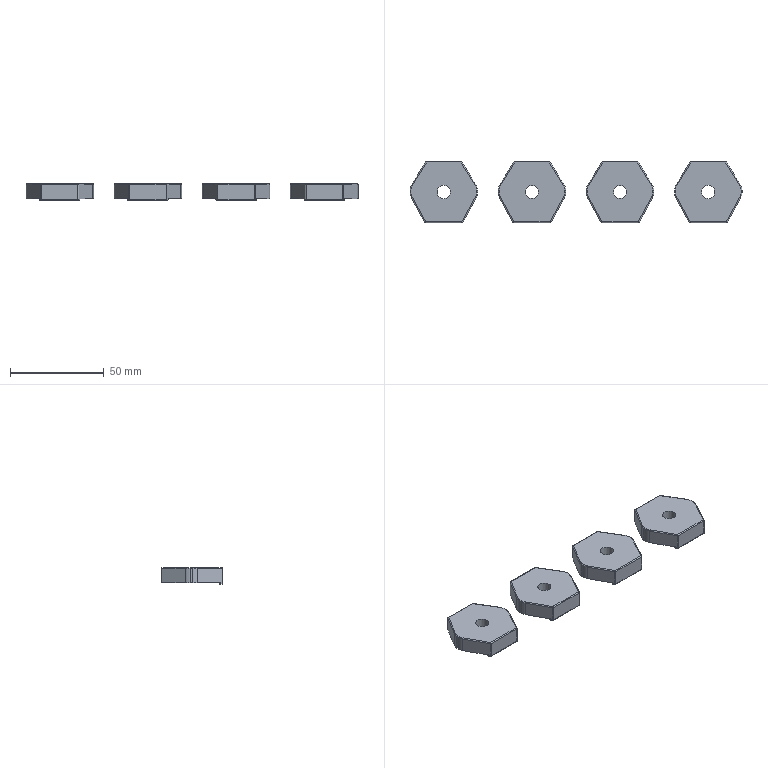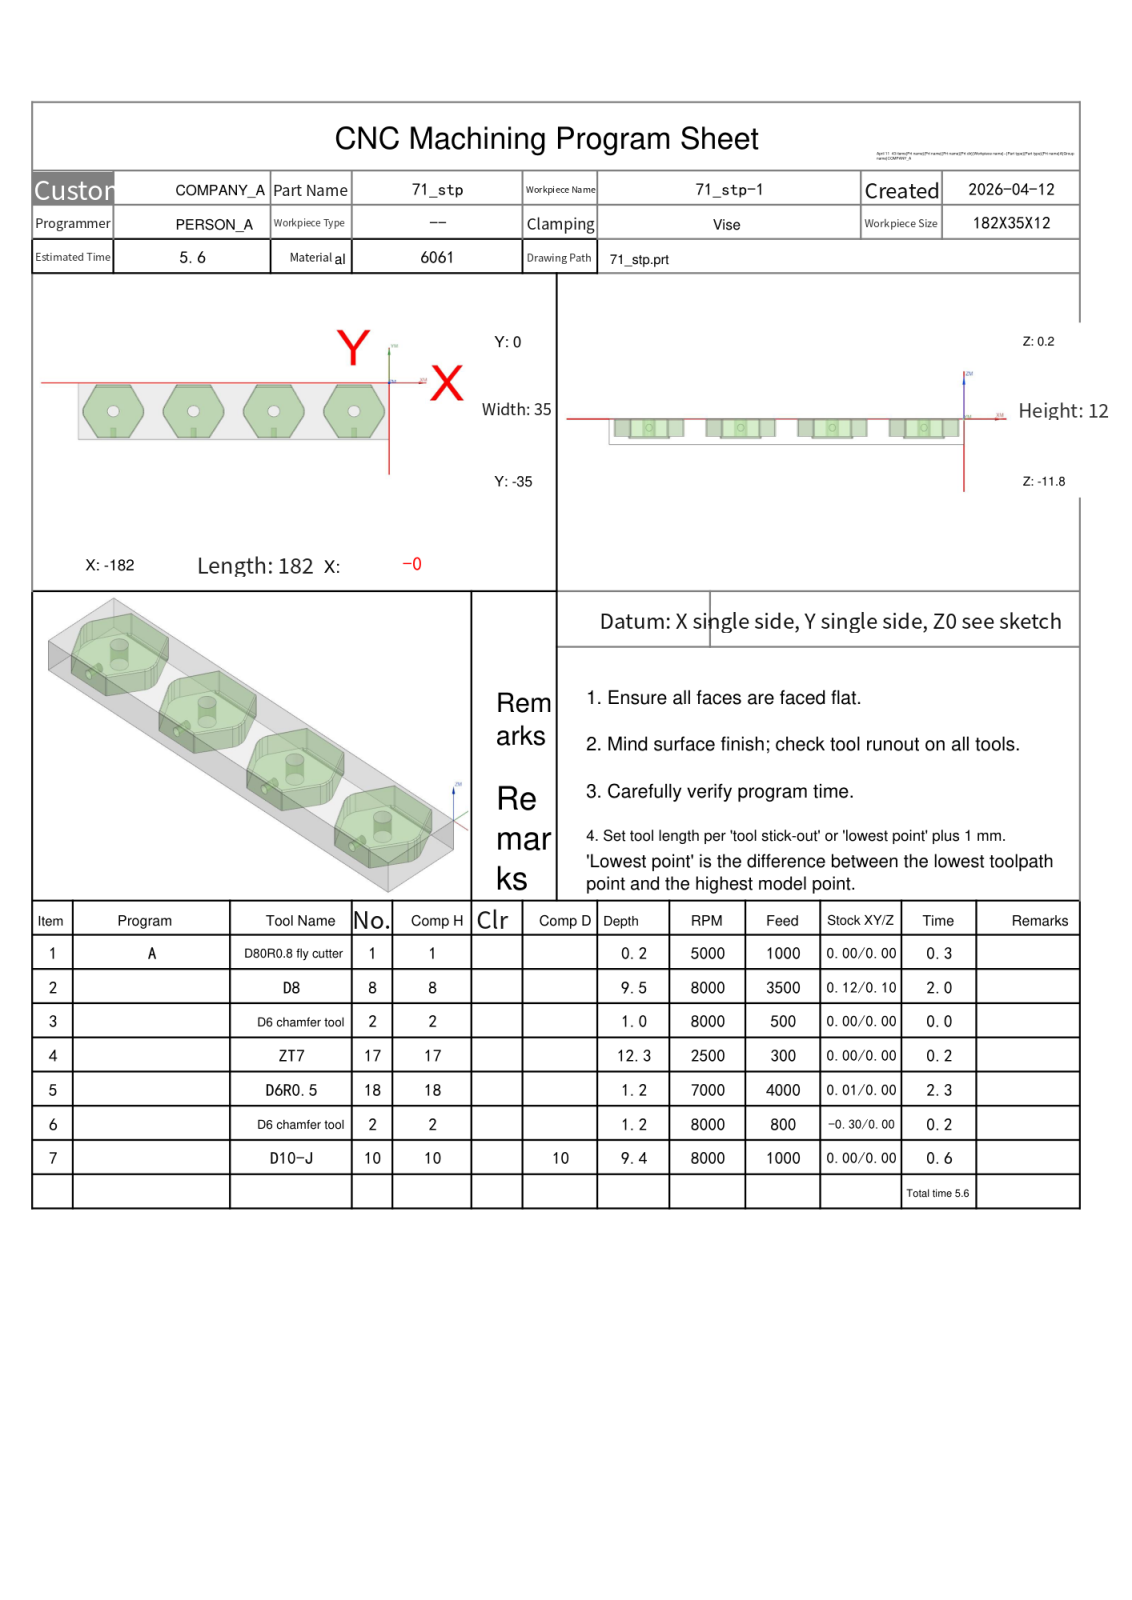NC program | NX | posted by the shop | part box 177 x 33 x 9 mm
Lines 34 to 853 of 15773:
N2 T08 M06
(D8  D=8. R=0. H=08 ce=0.12 di=0.10)
(MAX_Z=20. MIN_Z=-9.3 Time=2.03M)
G00 G90 G54 X-46.469 Y9.631 M03 S8000
G43 H08 Z20.
M08
Z-7.3
G01 X-46.451 Y9.533 Z-7.925 F3500.
X-46.433 Y9.435 Z-8.172
X-46.415 Y9.336 Z-8.354
X-46.396 Y9.238 Z-8.5
X-46.378 Y9.14 Z-8.623
X-46.36 Y9.041 Z-8.728
X-46.342 Y8.943 Z-8.82
X-46.324 Y8.845 Z-8.9
X-46.306 Y8.746 Z-8.97
X-46.287 Y8.648 Z-9.032
X-46.269 Y8.55 Z-9.086
X-46.251 Y8.451 Z-9.133
X-46.233 Y8.353 Z-9.174
X-46.215 Y8.255 Z-9.208
X-46.196 Y8.156 Z-9.236
X-46.178 Y8.058 Z-9.26
X-46.16 Y7.96 Z-9.277
X-46.142 Y7.861 Z-9.29
X-46.124 Y7.763 Z-9.297
X-46.105 Y7.665 Z-9.3
X-45.763 Y5.813
G03 X-45.53 Y5.517 I.405 J.08
X-42.414 Y5.012 I3.116 J9.363
G01 X-42.391
G03 X-34.679 Y4.895 I7.712 J253.536
X-32.981 Y4.9 I0.0 J253.653
G01 X-1.242 Y4.876
G02 X3.834 Y1.179 I-.204 J-5.613
X4.791 Y-4.109 I-15.027 J-5.451
X4.904 Y-11.94 I-270.442 J-7.831
X4.899 Y-13.588 I-270.556 J0.0
G01 X4.875 Y-33.767
G02 X1.064 Y-38.883 I-5.648 J.229
X-4.293 Y-39.8 I-5.462 J15.805
X-12.747 Y-39.907 I-8.454 J336.448
X-14.912 Y-39.9 I0.0 J336.554
G01 X-180.771 Y-39.875
G02 X-185.907 Y-36.005 I.244 J5.667
X-186.809 Y-30.524 I16.45 J5.52
X-186.9 Y-22.424 I358.144 J8.1
G01 X-186.899 Y-21.585
X-186.875 Y-1.225
G02 X-183.098 Y3.867 I5.635 J-.233
X-177.983 Y4.786 I5.357 J-15.119
X-169.888 Y4.907 I8.095 J-270.155
X-167.845 Y4.9 I0.0 J-270.276
G01 X-47.525 Y4.88
G03 X-36.07 Y4.289 I11.455 J110.869
X-34.358 Y4.303 I0.0 J111.459
G01 X-2.782 Y4.281
G02 X2.822 Y.462 I-.263 J-6.407
X4.101 Y-4.997 I-13.81 J-6.115
X4.319 Y-13.515 I-166.113 J-8.518
X4.299 Y-16.093 I-166.332 J0.0
G01 X4.273 Y-32.337
G02 X.456 Y-37.826 I-6.395 J.376
X-5.129 Y-39.111 I-6.168 J14.022
X-12.99 Y-39.311 I-7.861 J154.538
X-14.965 Y-39.298 I0.0 J154.738
G01 X-179.157 Y-39.283
G02 X-184.769 Y-35.572 I.183 J6.375
X-186.101 Y-30.002 I13.537 J6.183
X-186.313 Y-22.099 I147.476 J7.903
X-186.298 Y-20.047 I147.688 J0.0
X-186.324 Y-13.199 I932.526 J6.848
X-186.262 Y-2.503 I932.551 J0.0
X-182.47 Y2.818 I6.388 J-.54
X-176.892 Y4.109 I6.166 J-13.933
X-169.368 Y4.307 I7.524 J-142.898
X-167.716 Y4.298 I0.0 J-143.096
G01 X-48.656 Y4.275
G03 X-39.564 Y3.768 I19.57 J268.931
X-28.389 Y3.691 I11.176 J810.309
X-24.341 Y3.701 I0.0 J810.386
G01 X-4.162 Y3.679
G02 X2.13 Y-.639 I-.299 J-7.178
X3.495 Y-6.63 I-15.458 J-6.673
X3.71 Y-14.745 I-153.347 J-8.114
X3.698 Y-16.646 I-153.562 J0.0
X3.721 Y-22.166 I-646.386 J-5.52
X3.659 Y-31.125 I-646.409 J0.0
X-.568 Y-37.095 I-7.136 J.57
X-6.434 Y-38.479 I-6.628 J14.972
X-13.995 Y-38.704 I-7.56 J127.23
X-15.429 Y-38.695 I0.0 J127.454
G01 X-177.869 Y-38.676
G02 X-184.121 Y-34.381 I.319 J7.163
X-185.493 Y-28.391 I15.365 J6.672
X-185.711 Y-20.229 I153.286 J8.162
X-185.698 Y-18.255 I153.503 J0.0
X-185.723 Y-12.675 I620.518 J5.58
X-185.661 Y-3.896 I620.543 J0.0
X-181.441 Y2.091 I7.135 J-.548
X-175.399 Y3.493 I6.719 J-15.24
X-166.669 Y3.717 I8.73 J-169.523
X-164.123 Y3.698 I0.0 J-169.748
G01 X-49.623 Y3.675
G03 X-39.795 Y3.188 I46.086 J829.839
X-31.558 Y3.118 I8.237 J488.664
X-30.201 Y3.12 I0.0 J488.733
G01 X-5.734 Y3.089
X-5.73
G02 X1.522 Y-1.766 I0.0 J-7.844
X2.883 Y-7.949 I-16.932 J-6.968
X3.108 Y-16.247 I-153.023 J-8.298
X3.097 Y-18.084 I-153.248 J0.0
X3.116 Y-22.347 I-475.2 J-4.263
X3.058 Y-29.803 I-475.219 J0.0
X-1.706 Y-36.495 I-7.774 J.493
X-7.759 Y-37.868 I-6.923 J16.481
G01 X-10.659 Y-38.024
X-11.409 Y-38.12
X-175.683 Y-38.099
G02 X-176.12 Y-38.11 I-.437 J8.29
X-180.889 Y-36.604 I0.0 J8.302
X-184.211 Y-31.307 I5.976 J7.44
X-185.028 Y-24.203 I30.504 J7.104
G01 Y-24.17
G02 X-185.104 Y-13.157 I791.672 J11.013
X-185.065 Y-5.311 I791.749 J0.0
X-180.404 Y1.443 I7.76 J-.37
X-174.182 Y2.874 I7.039 J-16.362
G03 X-171.201 Y3.12 I-1.365 J34.726
G01 X-51.578 Y3.094
G02 X-41.401 Y2.65 I-11.338 J-376.674
G03 X-33.711 Y2.531 I7.69 J247.054
X-32.415 Y2.534 I0.0 J247.174
G02 X-30.298 Y3.107 I2.291 J-4.269
G03 X-32.525 Y2.487 I.219 J-5.098
G02 X-35.859 Y2.103 I-3.334 J14.267
X-36.319 Y2.11 I0.0 J14.652
X-48.557 Y2.523 I1.1 J213.807
G03 X-55.859 Y2.651 I-13.9 J-588.103
G01 X-56.551 Y2.949
X-57.767 Y3.12
G02 X-55.511 Y2.513 I-.263 J-5.475
G03 X-51.539 Y2.054 I4.131 J18.358
X-38.068 Y1.524 I23.165 J416.613
X-37.143 Y1.504 I.925 J21.92
X-33.407 Y1.825 I0.0 J21.939
G01 X-32.511 Y2.493
G02 X-33.72 Y1.652 I-4.216 J4.773
X-37.466 Y1.106 I-3.746 J12.559
X-37.794 Y1.11 I0.0 J13.106
X-49.056 Y1.461 I.153 J185.526
X-54.688 Y1.939 I.335 J37.41
X-55.421 Y2.462 I1.246 J2.524
G01 X-55.642 Y2.557
G02 X-54.763 Y1.937 I-1.218 J-2.657
G03 X-52.007 Y1.171 I3.286 J6.483
X-39.733 Y.542 I12.274 J119.512
X-37.401 Y.565 I0.0 J120.141
X-33.962 Y1.165 I-.011 J10.218
G01 X-33.535 Y1.7
X-33.347 Y1.849
G03 X-33.938 Y1.159 I1.796 J-2.136
G02 X-36.449 Y.31 I-2.939 J4.559
X-41.066 Y.075 I-4.617 J45.074
X-43.901 Y.163 I0.0 J45.309
X-52.223 Y.776 I1.511 J77.385
X-54.179 Y1.336 I1.063 J7.401
G03 X-54.789 Y1.957 I-2.181 J-1.534
G02 X-54.168 Y1.3 I-1.237 J-1.791
G03 X-51.671 Y.286 I3.24 J4.394
X-43.374 Y-.438 I8.951 J54.711
X-41.177 Y-.505 I2.196 J35.678
X-36.411 Y-.186 I0.0 J35.745
X-34.391 Y.502 I-.758 J5.538
G01 X-33.874 Y1.235
G02 X-34.512 Y.358 I-13.955 J9.477
X-37.332 Y-.654 I-3.401 J5.038
X-42.15 Y-.931 I-4.818 J41.8
X-45.107 Y-.827 I0.0 J42.076
X-51.964 Y-.05 I.649 J36.369
X-53.735 Y.7 I1.013 J4.858
G01 X-54.23 Y1.378
G03 X-51.829 Y-.435 I3.3 J1.872
X-45.617 Y-1.361 I6.951 J25.333
X-42.358 Y-1.494 I3.259 J40.079
X-37.719 Y-1.225 I0.0 J40.211
X-34.797 Y-.235 I-.727 J6.953
G01 X-34.355 Y.533
G02 X-36.116 Y-1.099 I-2.522 J.955
X-41.088 Y-1.898 I-4.972 J15.075
X-41.338 Y-1.896 I0.0 J15.873
X-42.823 Y-1.923 I-1.485 J40.915
X-50.606 Y-1.177 I0.0 J40.942
X-53.338 Y-.01 I1.208 J6.612
G01 X-53.723 Y.677
G03 X-51.726 Y-1.188 I3.021 J1.234
X-46.412 Y-2.288 I6.297 J17.03
X-42.884 Y-2.48 I3.528 J32.413
X-38.059 Y-2.121 I0.0 J32.605
X-35.216 Y-1.029 I-.953 J6.727
G01 X-34.741 Y-.179
G02 X-35.456 Y-1.309 I-3.581 J1.476
X-38.62 Y-2.562 I-4.02 J5.533
X-43.186 Y-2.898 I-4.566 J30.791
X-50.247 Y-2.087 I0.0 J31.128
X-52.926 Y-.794 I1.301 J6.116
G01 X-53.326 Y-.056
G03 X-51.112 Y-2.166 I3.415 J1.366
X-45.183 Y-3.347 I6.562 J17.469
X-42.999 Y-3.446 I2.184 J23.958
X-37.991 Y-2.919 I0.0 J24.058
X-35.644 Y-1.846 I-.982 J5.25
G01 X-35.187 Y-1.002
G02 X-36.024 Y-2.267 I-3.53 J1.426
X-39.542 Y-3.576 I-4.365 J6.353
X-43.323 Y-3.859 I-3.781 J25.068
X-50.068 Y-2.946 I0.0 J25.352
X-52.434 Y-1.701 I1.645 J5.999
G01 X-52.892 Y-.857
G03 X-51.875 Y-2.352 I4.074 J1.675
X-47.986 Y-3.915 I5.233 J7.404
X-43.392 Y-4.381 I4.594 J22.38
X-38.543 Y-3.861 I0.0 J22.847
X-36.126 Y-2.736 I-1.063 J5.442
G01 X-35.669 Y-1.892
G02 X-36.509 Y-3.168 I-3.629 J1.474
X-40.156 Y-4.534 I-4.473 J6.392
X-43.452 Y-4.79 I-3.296 J21.024
X-49.853 Y-3.805 I0.0 J21.281
X-51.93 Y-2.632 I1.816 J5.64
G01 X-52.387 Y-1.788
G03 X-51.392 Y-3.276 I4.284 J1.787
X-47.5 Y-4.881 I5.221 J7.14
X-43.5 Y-5.296 I4.001 J19.067
X-38.748 Y-4.708 I0.0 J19.482
X-36.621 Y-3.649 I-1.175 J5.025
G01 X-36.164 Y-2.805
G02 X-37.012 Y-4.094 I-3.647 J1.476
X-40.684 Y-5.469 I-4.484 J6.385
X-43.556 Y-5.695 I-2.872 J18.077
X-49.594 Y-4.671 I0.0 J18.304
X-51.41 Y-3.59 I1.963 J5.367
G01 X-51.896 Y-2.694
G03 X-50.975 Y-4.145 I4.966 J2.135
X-47.318 Y-5.771 I4.983 J6.283
X-43.586 Y-6.188 I3.732 J16.465
X-38.949 Y-5.539 I0.0 J16.883
X-37.125 Y-4.579 I-1.349 J4.772
G01 X-36.639 Y-3.682
G02 X-37.394 Y-4.913 I-4.591 J1.967
X-40.774 Y-6.317 I-4.241 J5.442
X-43.639 Y-6.577 I-2.865 J15.657
X-49.346 Y-5.519 I0.0 J15.917
X-50.888 Y-4.555 I2.104 J5.08
G01 X-51.374 Y-3.658
G03 X-50.446 Y-5.114 I4.899 J2.097
X-46.672 Y-6.741 I4.945 J6.281
X-43.641 Y-7.059 I3.031 J14.248
X-39.062 Y-6.321 I0.0 J14.567
X-37.625 Y-5.501 I-1.449 J4.21
G01 X-37.139 Y-4.604
G02 X-37.901 Y-5.842 I-4.494 J1.915
X-41.275 Y-7.22 I-4.154 J5.349
X-43.715 Y-7.437 I-2.44 J13.597
X-49.173 Y-6.313 I0.0 J13.814
X-50.368 Y-5.514 I2.349 J4.808
G01 X-50.854 Y-4.617
G03 X-49.922 Y-6.075 I4.816 J2.052
X-46.137 Y-7.662 I4.796 J6.127
X-43.675 Y-7.904 I2.462 J12.437
X-39.266 Y-7.113 I0.0 J12.678
X-38.118 Y-6.411 I-1.394 J3.573
G01 X-37.632 Y-5.514
G02 X-38.389 Y-6.748 I-4.566 J1.953
X-41.762 Y-8.099 I-4.037 J5.196
X-43.781 Y-8.268 I-2.019 J11.946
X-48.871 Y-7.147 I0.0 J12.115
X-49.856 Y-6.459 I2.659 J4.856
G01 X-50.314 Y-5.615
G03 X-49.29 Y-7.122 I4.133 J1.705
X-45.019 Y-8.63 I4.774 J6.717
X-43.622 Y-8.723 I1.397 J10.414
X-39.305 Y-7.796 I0.0 J10.507
X-38.61 Y-7.32 I-1.855 J3.452
G01 X-38.124 Y-6.423
G02 X-38.889 Y-7.659 I-4.322 J1.82
X-42.349 Y-8.964 I-3.932 J5.183
X-43.857 Y-9.073 I-1.508 J10.379
X-48.634 Y-7.922 I0.0 J10.488
X-49.352 Y-7.389 I5.004 J7.492
G01 X-49.809 Y-6.545
G03 X-48.804 Y-8.031 I4.08 J1.678
X-44.533 Y-9.462 I4.501 J6.348
X-43.6 Y-9.51 I.932 J8.926
X-39.526 Y-8.532 I0.0 J8.974
G01 X-39.088 Y-8.202
X-38.631 Y-7.358
G02 X-39.361 Y-8.533 I-4.078 J1.72
X-42.689 Y-9.765 I-3.7 J4.88
X-43.927 Y-9.851 I-1.238 J8.923
X-48.43 Y-8.645 I0.0 J9.008
G01 X-48.862 Y-8.293
X-49.32 Y-7.449
G03 X-48.42 Y-8.838 I4.339 J1.826
X-44.469 Y-10.224 I4.147 J5.495
X-43.643 Y-10.267 I.826 J7.886
X-39.862 Y-9.308 I0.0 J7.929
G01 X-39.553 Y-9.059
X-39.095 Y-8.215
G02 X-39.827 Y-9.388 I-3.946 J1.648
X-43.295 Y-10.554 I-3.536 J4.772
X-44.004 Y-10.587 I-.708 J7.74
X-48.065 Y-9.441 I0.0 J7.772
G01 X-48.39 Y-9.165
X-48.819 Y-8.374
G03 X-47.851 Y-9.785 I3.72 J1.514
X-43.946 Y-10.993 I3.905 J5.706
X-43.309 Y-10.963 I0.0 J6.914
X-40.043 Y-9.935 I-.072 J5.934
G01 X-39.567 Y-9.085
G02 X-40.289 Y-10.22 I-3.505 J1.434
X-43.588 Y-11.285 I-3.299 J4.576
G01 X-43.786 Y-11.281
G02 X-44.112 Y-11.29 I-.326 J6.425
X-47.878 Y-10.072 I0.0 J6.433
G01 X-48.336 Y-9.264
G03 X-47.381 Y-10.624 I3.39 J1.365
X-43.826 Y-11.688 I3.555 J5.407
X-40.577 Y-10.814 I0.0 J6.471
X-39.996 Y-9.877 I-2.331 J2.095
G02 X-40.72 Y-11.008 I-3.351 J1.349
X-43.785 Y-11.972 I-3.065 J4.389
X-44.403 Y-11.936 I0.0 J5.354
X-47.505 Y-10.797 I.098 J5.062
G01 X-47.906 Y-10.059
G03 X-46.929 Y-11.423 I3.215 J1.271
X-43.849 Y-12.335 I3.079 J4.743
X-40.915 Y-11.514 I0.0 J5.655
G01 X-40.43 Y-10.677
G02 X-41.125 Y-11.75 I-3.065 J1.224
X-43.907 Y-12.606 I-2.782 J4.092
X-44.897 Y-12.506 I0.0 J4.948
X-47.1 Y-11.545 I.488 J4.122
G01 X-47.472 Y-10.859
G03 X-46.432 Y-12.221 I2.862 J1.107
X-43.872 Y-12.935 I2.561 J4.234
X-41.285 Y-12.205 I0.0 J4.948
G01 X-40.835 Y-11.426
G02 X-41.618 Y-12.53 I-2.498 J.941
X-43.974 Y-13.185 I-2.356 J3.91
X-46.681 Y-12.296 I0.0 J4.565
G01 X-47.065 Y-11.61
G03 X-44.869 Y-13.368 I2.586 J.98
X-43.854 Y-13.495 I1.015 J3.964
X-41.604 Y-12.821 I0.0 J4.092
G01 X-41.232 Y-12.158
G02 X-41.945 Y-13.156 I-2.177 J.802
X-43.978 Y-13.72 I-2.033 J3.38
X-46.361 Y-12.919 I0.0 J3.944
G01 X-46.681 Y-12.318
G03 X-45.962 Y-13.363 I2.496 J.948
X-43.9 Y-14.006 I2.062 J2.986
X-41.852 Y-13.373 I0.0 J3.629
G01 X-41.54 Y-12.735
G02 X-43.049 Y-14.086 I-1.796 J.489
X-43.978 Y-14.216 I-.929 J3.253
X-46.138 Y-13.437 I0.0 J3.383
G01 X-46.392 Y-12.888
G03 X-44.68 Y-14.369 I2.016 J.601
X-43.884 Y-14.472 I.796 J2.997
X-42.084 Y-13.897 I0.0 J3.101
G01 X-41.803 Y-13.321
G02 X-43.2 Y-14.559 I-1.647 J.451
X-43.99 Y-14.669 I-.79 J2.8
X-45.923 Y-13.933 I0.0 J2.909
G01 X-46.16 Y-13.412
G03 X-44.368 Y-14.855 I1.935 J.569
X-43.859 Y-14.906 I.509 J2.481
X-42.204 Y-14.291 I0.0 J2.533
G01 X-42.029 Y-13.825
G02 X-43.101 Y-14.929 I-1.362 J.251
X-43.981 Y-15.085 I-.879 J2.401
X-45.796 Y-14.329 I0.0 J2.557
G01 X-45.919 Y-13.956
G03 X-44.626 Y-15.189 I1.541 J.321
X-43.904 Y-15.301 I.722 J2.276
X-42.321 Y-14.7 I0.0 J2.388
G01 X-42.146 Y-14.18
G02 X-43.219 Y-15.337 I-1.327 J.154
X-43.983 Y-15.466 I-.764 J2.192
X-45.696 Y-14.712 I0.0 J2.321
G01 X-45.82 Y-14.295
G03 X-44.504 Y-15.584 I1.524 J.24
X-43.903 Y-15.669 I.601 J2.072
X-42.412 Y-15.071 I0.0 J2.158
G01 X-42.259 Y-14.586
G02 X-43.347 Y-15.722 I-1.287 J.144
X-43.99 Y-15.82 I-.643 J2.05
X-45.596 Y-15.098 I0.0 J2.149
G01 X-45.716 Y-14.689
G03 X-44.409 Y-15.951 I1.478 J.223
X-43.897 Y-16.02 I.512 J1.861
X-42.497 Y-15.419 I0.0 J1.931
G01 X-42.381 Y-15.023
G02 X-43.366 Y-16.058 I-1.182 J.139
X-44.006 Y-16.167 I-.64 J1.813
X-45.514 Y-15.437 I0.0 J1.923
G01 X-45.618 Y-15.06
G03 X-44.212 Y-16.31 I1.456 J.222
X-43.872 Y-16.343 I.34 J1.705
X-42.52 Y-15.699 I0.0 J1.738
G01 X-42.445 Y-15.255
X-42.444 Y-15.3
G02 X-43.264 Y-16.336 I-1.065 J0.0
X-43.982 Y-16.48 I-.718 J1.721
X-45.47 Y-15.739 I0.0 J1.865
G01 X-45.526 Y-15.408
G03 X-44.622 Y-16.518 I1.172 J.031
X-43.934 Y-16.654 I.688 J1.678
X-42.57 Y-16.035 I0.0 J1.814
G01 X-42.488 Y-15.612
Y-15.632
G02 X-43.283 Y-16.645 I-1.044 J0.0
X-43.985 Y-16.791 I-.703 J1.621
X-45.453 Y-16.008 I0.0 J1.767
G01 X-45.503 Y-15.638
Y-15.649
G03 X-44.48 Y-16.866 I1.236 J0.0
X-43.922 Y-16.961 I.558 J1.596
X-42.593 Y-16.316 I0.0 J1.691
G01 X-42.526 Y-15.926
G02 X-43.481 Y-17.005 I-1.103 J.014
X-43.995 Y-17.084 I-.514 J1.641
X-45.419 Y-16.329 I0.0 J1.719
G01 X-45.471 Y-15.953
Y-15.96
G03 X-44.406 Y-17.179 I1.23 J0.0
X-43.919 Y-17.253 I.488 J1.552
X-42.63 Y-16.62 I0.0 J1.627
G01 X-42.556 Y-16.171
Y-16.205
G02 X-43.527 Y-17.307 I-1.111 J0.0
X-44.017 Y-17.384 I-.49 J1.527
X-45.401 Y-16.591 I0.0 J1.604
G01 X-45.441 Y-16.257
Y-16.269
G03 X-44.382 Y-17.471 I1.212 J0.0
X-43.913 Y-17.544 I.469 J1.471
X-42.644 Y-16.879 I0.0 J1.544
G01 X-42.596 Y-16.504
X-42.595 Y-16.567
G02 X-43.352 Y-17.532 I-.993 J0.0
X-43.993 Y-17.664 I-.641 J1.494
X-45.364 Y-16.912 I0.0 J1.626
G01 X-45.406 Y-16.607
G03 X-44.285 Y-17.775 I1.214 J.043
X-43.913 Y-17.821 I.372 J1.477
X-42.656 Y-17.159 I0.0 J1.523
G01 X-42.616 Y-16.755
X-42.611 Y-16.854
G02 X-43.379 Y-17.818 I-.99 J0.0
X-44. Y-17.947 I-.621 J1.428
X-45.363 Y-17.143 I0.0 J1.557
G01 X-45.381 Y-16.895
Y-16.929
G03 X-44.55 Y-17.976 I1.076 J0.0
X-43.938 Y-18.103 I.612 J1.412
X-42.666 Y-17.431 I0.0 J1.539
G01 X-42.628 Y-17.033
X-42.623 Y-17.132
G02 X-43.38 Y-18.094 I-.99 J0.0
X-43.992 Y-18.218 I-.611 J1.451
X-45.351 Y-17.439 I0.0 J1.575
G01 X-45.375 Y-17.115
X-45.378 Y-17.192
G03 X-44.527 Y-18.257 I1.092 J0.0
X-43.94 Y-18.374 I.587 J1.411
X-42.679 Y-17.709 I0.0 J1.529
G01 X-42.64 Y-17.306
X-42.636 Y-17.387
G02 X-43.518 Y-18.411 I-1.036 J0.0
X-44. Y-18.488 I-.482 J1.48
X-45.343 Y-17.719 I0.0 J1.557
G01 X-45.368 Y-17.391
X-45.371 Y-17.465
G03 X-44.507 Y-18.536 I1.095 J0.0
X-43.93 Y-18.653 I.577 J1.361
X-42.675 Y-17.955 I0.0 J1.478
G01 X-42.65 Y-17.555
X-42.643 Y-17.677
G02 X-43.475 Y-18.667 I-1.006 J0.0
X-44.011 Y-18.766 I-.536 J1.407
X-45.346 Y-17.956 I0.0 J1.505
G01 X-45.361 Y-17.665
X-45.363 Y-17.726
G03 X-44.403 Y-18.838 I1.124 J0.0
X-43.927 Y-18.917 I.475 J1.399
X-42.664 Y-18.205 I0.0 J1.477
G01 X-42.653 Y-17.843
X-42.642 Y-17.986
G02 X-43.331 Y-18.883 I-.928 J0.0
X-43.997 Y-19.037 I-.666 J1.361
X-45.342 Y-18.219 I0.0 J1.515
G01 X-45.354 Y-17.954
X-45.357 Y-18.036
G03 X-44.539 Y-19.064 I1.055 J0.0
X-43.941 Y-19.187 I.599 J1.386
X-42.653 Y-18.467 I0.0 J1.51
G01 X-42.642 Y-18.103
X-42.632 Y-18.244
G02 X-43.326 Y-19.154 I-.943 J0.0
X-43.985 Y-19.299 I-.659 J1.425
X-45.349 Y-18.507 I0.0 J1.57
G01 X-45.358 Y-18.202
X-45.364 Y-18.309
G03 X-44.572 Y-19.321 I1.043 J0.0
X-43.938 Y-19.462 I.635 J1.359
X-42.638 Y-18.711 I0.0 J1.5
G01 X-42.631 Y-18.369
X-42.622 Y-18.5
G02 X-43.342 Y-19.436 I-.968 J0.0
X-43.986 Y-19.575 I-.644 J1.42
X-45.369 Y-18.736 I0.0 J1.559
G01 X-45.37 Y-18.401
X-45.382 Y-18.562
G03 X-44.61 Y-19.58 I1.057 J0.0
X-43.944 Y-19.732 I.666 J1.384
X-42.63 Y-18.991 I0.0 J1.536
G01 X-42.623 Y-18.556
G02 X-42.603 Y-18.755 I-.953 J-.2
X-43.286 Y-19.685 I-.973 J0.0
X-43.99 Y-19.853 I-.704 J1.388
X-45.387 Y-18.982 I0.0 J1.556
G01 X-45.384 Y-18.664
X-45.396 Y-18.823
G03 X-44.616 Y-19.855 I1.073 J0.0
X-43.948 Y-20.004 I.668 J1.423
X-42.603 Y-19.244 I0.0 J1.572
G01 X-42.611 Y-18.855
G02 X-42.588 Y-19.058 I-.897 J-.202
X-43.214 Y-19.929 I-.92 J0.0
X-43.981 Y-20.126 I-.767 J1.396
X-45.4 Y-19.258 I0.0 J1.593
G01 X-45.399 Y-18.929
X-45.411 Y-19.089
G03 X-44.644 Y-20.123 I1.08 J0.0
X-43.944 Y-20.288 I.7 J1.402
X-42.563 Y-19.461 I0.0 J1.567
G01 X-42.588 Y-19.031
G02 X-42.549 Y-19.299 I-.907 J-.268
X-43.16 Y-20.183 I-.946 J0.0
X-43.978 Y-20.406 I-.818 J1.395
X-45.424 Y-19.512 I0.0 J1.617
G01 X-45.413 Y-19.174
X-45.431 Y-19.37
G03 X-44.712 Y-20.374 I1.061 J0.0
X-43.949 Y-20.562 I.763 J1.456
X-42.542 Y-19.768 I0.0 J1.644
G01 X-42.539 Y-19.603
G03 X-42.547 Y-19.347 I-3.865 J0.0
G02 X-42.52 Y-19.572 I-.919 J-.225
X-43.129 Y-20.456 I-.946 J0.0
X-43.973 Y-20.687 I-.844 J1.423
X-45.458 Y-19.763 I0.0 J1.655
G01 X-45.442 Y-19.428
G03 X-45.467 Y-19.652 I1.01 J-.224
X-44.803 Y-20.618 I1.035 J0.0
X-43.951 Y-20.848 I.852 J1.461
X-42.511 Y-20.044 I0.0 J1.692
X-42.502 Y-19.839 I-2.435 J.206
X-42.512 Y-19.617 I-2.444 J0.0
G02 X-42.485 Y-19.845 I-.914 J-.228
X-43.048 Y-20.708 I-.942 J0.0
X-43.969 Y-20.98 I-.92 J1.424
X-45.506 Y-20. I0.0 J1.695
G01 X-45.475 Y-19.623
G03 X-45.512 Y-19.902 I1.031 J-.279
X-44.852 Y-20.889 I1.068 J0.0
X-43.949 Y-21.149 I.904 J1.444
X-42.462 Y-20.276 I0.0 J1.703
G01 X-42.476 Y-19.897
G02 X-42.451 Y-20.116 I-.942 J-.22
X-43.029 Y-21.002 I-.968 J0.0
X-43.968 Y-21.276 I-.939 J1.469
X-45.55 Y-20.265 I0.0 J1.744
G01 X-45.52 Y-19.888
G03 X-45.557 Y-20.169 I1.052 J-.281
X-44.903 Y-21.167 I1.089 J0.0
X-43.951 Y-21.443 I.952 J1.505
X-42.437 Y-20.6 I0.0 J1.781
G01 X-42.43 Y-20.413
G03 X-42.446 Y-20.13 I-2.526 J0.0
G02 X-42.41 Y-20.394 I-.934 J-.263
X-42.946 Y-21.261 I-.97 J0.0
X-43.968 Y-21.582 I-1.022 J1.469
X-45.6 Y-20.527 I0.0 J1.79
G01 X-45.567 Y-20.161
G03 X-45.604 Y-20.445 I1.071 J-.285
X-44.962 Y-21.45 I1.108 J0.0
X-43.955 Y-21.754 I1.006 J1.513
X-42.369 Y-20.823 I0.0 J1.817
G01 X-42.36 Y-20.691
G03 X-42.415 Y-20.369 I-.959 J0.0
G02 X-42.351 Y-20.704 I-.836 J-.335
X-42.819 Y-21.494 I-.9 J0.0
X-43.966 Y-21.886 I-1.147 J1.479
X-45.636 Y-20.861 I0.0 J1.872
G01 Y-20.822
G02 X-45.609 Y-20.412 I3.191 J0.0
G03 X-45.65 Y-20.717 I1.114 J-.304
X-44.963 Y-21.773 I1.155 J0.0
X-43.95 Y-22.072 I1.014 J1.568
X-42.294 Y-21.068 I0.0 J1.867
G01 X-42.284 Y-20.926
G03 X-42.367 Y-20.527 I-1.003 J0.0
G02 X-42.272 Y-20.944 I-.871 J-.418
X-42.739 Y-21.771 I-.966 J0.0
X-43.961 Y-22.211 I-1.222 J1.477
X-45.685 Y-21.132 I0.0 J1.917
G01 X-45.71 Y-20.942
G02 X-45.65 Y-20.649 I.743 J0.0
G03 X-45.722 Y-21.035 I.99 J-.386
X-45.201 Y-21.95 I1.062 J0.0
X-43.953 Y-22.395 I1.248 J1.528
X-42.222 Y-21.366 I0.0 J1.972
G01 X-42.201 Y-21.181
G03 X-42.266 Y-20.857 I-.827 J0.0
G02 X-42.193 Y-21.228 I-.899 J-.371
X-42.636 Y-22.044 I-.972 J0.0
X-43.958 Y-22.535 I-1.322 J1.535
X-45.728 Y-21.494 I0.0 J2.026
X-45.797 Y-21.185 I.651 J.309
X-45.718 Y-20.856 I.721 J0.0
G03 X-45.809 Y-21.296 I1.02 J-.44
X-45.296 Y-22.232 I1.111 J0.0
X-43.952 Y-22.733 I1.344 J1.554
X-42.148 Y-21.662 I0.0 J2.055
X-42.115 Y-21.434 I-.778 J.229
X-42.201 Y-21.071 I-.81 J0.0
G02 X-42.104 Y-21.502 I-.909 J-.432
X-42.525 Y-22.321 I-1.006 J0.0
X-43.955 Y-22.878 I-1.43 J1.558
X-45.82 Y-21.76 I0.0 J2.115
X-45.886 Y-21.456 I.673 J.304
X-45.806 Y-21.122 I.738 J0.0
G03 X-45.9 Y-21.575 I1.044 J-.453
X-45.424 Y-22.501 I1.138 J0.0
X-43.949 Y-23.078 I1.475 J1.593
X-42.097 Y-22.039 I0.0 J2.171
X-42.023 Y-21.716 I-.667 J.323
X-42.112 Y-21.363 I-.741 J0.0
G02 X-42.018 Y-21.798 I-.95 J-.435
X-42.437 Y-22.635 I-1.045 J0.0
X-43.954 Y-23.231 I-1.517 J1.631
X-45.896 Y-22.093 I0.0 J2.228
X-45.982 Y-21.737 I.695 J.356
X-45.883 Y-21.355 I.781 J0.0
G03 X-45.995 Y-21.861 I1.083 J-.506
X-45.513 Y-22.821 I1.195 J0.0
X-43.95 Y-23.445 I1.562 J1.643
X-41.994 Y-22.324 I0.0 J2.267
X-41.935 Y-22.01 I-.795 J.313
X-42.04 Y-21.6 I-.854 J0.0
G02 X-41.921 Y-22.097 I-.981 J-.498
X-42.369 Y-22.983 I-1.1 J0.0
X-43.952 Y-23.599 I-1.583 J1.727
X-45.976 Y-22.438 I0.0 J2.343
X-46.083 Y-22.042 I.68 J.396
X-45.983 Y-21.659 I.787 J0.0
G03 X-46.09 Y-22.166 I1.158 J-.508
X-45.562 Y-23.194 I1.264 J0.0
X-43.947 Y-23.816 I1.615 J1.786
X-41.949 Y-22.751 I0.0 J2.408
X-41.804 Y-22.306 I-.614 J.445
X-41.965 Y-21.839 I-.759 J0.0
G02 X-41.786 Y-22.407 I-.811 J-.568
X-42.081 Y-23.112 I-.991 J0.0
X-43.955 Y-23.981 I-1.874 J1.587
X-46.058 Y-22.795 I0.0 J2.456
X-46.192 Y-22.356 I.647 J.439
X-46.081 Y-21.954 I.782 J0.0
G03 X-46.229 Y-22.495 I.91 J-.541
X-45.963 Y-23.197 I1.058 J0.0
X-43.939 Y-24.206 I2.023 J1.524
X-41.83 Y-23.075 I0.0 J2.533
X-41.672 Y-22.593 I-.659 J.483
X-41.829 Y-22.111 I-.817 J0.0
G02 X-41.649 Y-22.697 I-.863 J-.586
X-41.936 Y-23.415 I-1.043 J0.0
X-43.953 Y-24.382 I-2.017 J1.622
X-46.188 Y-23.099 I0.0 J2.588
X-46.325 Y-22.633 I.726 J.466
X-46.19 Y-22.169 I.863 J0.0
G03 X-46.364 Y-22.786 I1.01 J-.618
X-46.041 Y-23.599 I1.184 J0.0
X-43.939 Y-24.617 I2.102 J1.663
X-41.686 Y-23.388 I0.0 J2.68
X-41.526 Y-22.885 I-.715 J.503
X-41.711 Y-22.348 I-.874 J0.0
G02 X-41.503 Y-23.005 I-.935 J-.657
X-41.838 Y-23.813 I-1.142 J0.0
X-43.947 Y-24.8 I-2.109 J1.758
X-46.323 Y-23.43 I0.0 J2.745
X-46.471 Y-22.927 I.787 J.504
X-46.305 Y-22.397 I.934 J0.0
G03 X-46.509 Y-23.094 I1.092 J-.697
X-46.14 Y-24. I1.296 J0.0
X-43.939 Y-25.049 I2.2 J1.783
X-41.508 Y-23.668 I0.0 J2.832
X-41.37 Y-23.206 I-.708 J.462
X-41.528 Y-22.713 I-.846 J0.0
G02 X-41.34 Y-23.325 I-.903 J-.612
X-41.584 Y-24.012 I-1.091 J0.0
X-43.949 Y-25.238 I-2.365 J1.669
X-46.491 Y-23.728 I0.0 J2.895
X-46.626 Y-23.24 I.814 J.488
X-46.463 Y-22.707 I.949 J0.0
G03 X-46.669 Y-23.418 I1.124 J-.711
X-46.333 Y-24.303 I1.33 J0.0
X-43.935 Y-25.492 I2.398 J1.821
X-41.362 Y-24.046 I0.0 J3.011
X-41.206 Y-23.544 I-.729 J.502
X-41.367 Y-23.035 I-.885 J0.0
G02 X-41.171 Y-23.661 I-.899 J-.626
X-41.395 Y-24.325 I-1.095 J0.0
X-43.95 Y-25.691 I-2.555 J1.708
X-46.638 Y-24.109 I0.0 J3.073
X-46.79 Y-23.576 I.854 J.532
X-46.621 Y-23.018 I1.007 J0.0
G03 X-46.841 Y-23.757 I1.128 J-.739
X-46.535 Y-24.613 I1.348 J0.0
X-43.926 Y-25.948 I2.608 J1.881
X-41.251 Y-24.517 I0.0 J3.216
X-41.033 Y-23.843 I-.933 J.674
X-41.07 Y-23.551 I-1.151 J0.0
G01 X-41.227 Y-23.295
G02 X-40.983 Y-23.99 I-.87 J-.695
X-41.175 Y-24.615 I-1.114 J0.0
X-43.937 Y-26.162 I-2.761 J1.691
X-45.187 Y-25.911 I0.0 J3.238
X-46.973 Y-23.775 I.757 J2.448
X-46.765 Y-23.281 I1.101 J-.174
G03 X-47.033 Y-24.092 I1.091 J-.811
X-46.756 Y-24.914 I1.359 J0.0
X-43.919 Y-26.431 I2.837 J1.895
X-41.07 Y-24.896 I0.0 J3.412
X-40.839 Y-24.166 I-1.043 J.731
X-40.873 Y-23.874 I-1.273 J0.0
G01 X-41.061 Y-23.567
G02 X-40.784 Y-24.323 I-.894 J-.756
X-40.957 Y-24.936 I-1.171 J0.0
X-43.887 Y-26.648 I-2.93 J1.65
X-44.684 Y-26.553 I0.0 J3.363
X-47.12 Y-24.469 I.46 J3.003
X-47.169 Y-24.173 I.88 J.296
X-46.929 Y-23.549 I.929 J0.0
G03 X-47.23 Y-24.442 I1.169 J-.892
X-46.925 Y-25.339 I1.471 J0.0
X-43.916 Y-26.934 I3.009 J2.041
X-40.886 Y-25.307 I0.0 J3.636
X-40.634 Y-24.512 I-1.132 J.795
X-40.667 Y-24.212 I-1.383 J0.0
G01 X-40.854 Y-23.905
G02 X-40.576 Y-24.699 I-.99 J-.793
X-40.796 Y-25.413 I-1.268 J0.0
X-43.896 Y-27.159 I-3.1 J1.88
X-44.899 Y-27.017 I0.0 J3.626
X-47.328 Y-24.82 I.624 J3.131
X-47.376 Y-24.521 I.905 J.298
X-47.135 Y-23.888 I.952 J0.0
G03 X-47.445 Y-24.789 I1.155 J-.901
X-47.21 Y-25.585 I1.465 J0.0
X-43.935 Y-27.453 I3.275 J1.936
X-42.808 Y-27.282 I0.0 J3.804
X-40.42 Y-24.985 I-.659 J3.076
G01 X-40.406 Y-24.835
G03 X-40.637 Y-24.262 I-.828 J0.0
G02 X-40.354 Y-25.069 I-1.01 J-.807
X-40.551 Y-25.754 I-1.293 J0.0
X-43.846 Y-27.682 I-3.295 J1.852
X-44.511 Y-27.623 I0.0 J3.78
X-47.477 Y-25.433 I.344 J3.571
X-47.592 Y-24.938 I1.014 J.495
X-47.349 Y-24.238 I1.129 J0.0
G03 X-47.661 Y-25.181 I1.268 J-.943
X-47.379 Y-26.082 I1.58 J0.0
X-43.934 Y-27.991 I3.445 J2.155
X-42.78 Y-27.823 I0.0 J4.063
X-40.235 Y-25.575 I-.726 J3.387
X-40.173 Y-25.24 I-.875 J.335
X-40.44 Y-24.585 I-.937 J0.0
G02 X-40.124 Y-25.456 I-1.042 J-.871
X-40.323 Y-26.163 I-1.358 J0.0
X-43.788 Y-28.218 I-3.466 J1.895
X-44.106 Y-28.205 I0.0 J3.95
X-47.642 Y-25.99 I.007 J3.942
X-47.804 Y-25.282 I1.467 J.708
X-47.762 Y-24.916 I1.629 J0.0
G01 X-47.544 Y-24.558
G03 X-47.892 Y-25.566 I1.284 J-1.008
X-47.638 Y-26.442 I1.632 J0.0
X-43.974 Y-28.543 I3.664 J2.144
X-43.192 Y-28.471 I0.0 J4.245
X-40.05 Y-26.15 I-.409 J3.841
X-39.938 Y-25.674 I-.952 J.475
X-40.206 Y-24.968 I-1.064 J0.0
G02 X-39.884 Y-25.853 I-1.057 J-.886
X-40.063 Y-26.531 I-1.379 J0.0
X-43.681 Y-28.768 I-3.646 J1.853
X-44.054 Y-28.784 I-.373 J4.256
X-47.839 Y-26.494 I0.0 J4.272
X-48.037 Y-25.681 I1.571 J.813
X-47.995 Y-25.298 I1.769 J0.0
G01 X-47.776 Y-24.94
G03 X-48.132 Y-25.97 I1.313 J-1.03
X-47.902 Y-26.816 I1.669 J0.0
X-44.037 Y-29.109 I3.864 J2.111
X-43.656 Y-29.092 I0.0 J4.404
X-39.862 Y-26.724 I-.025 J4.263